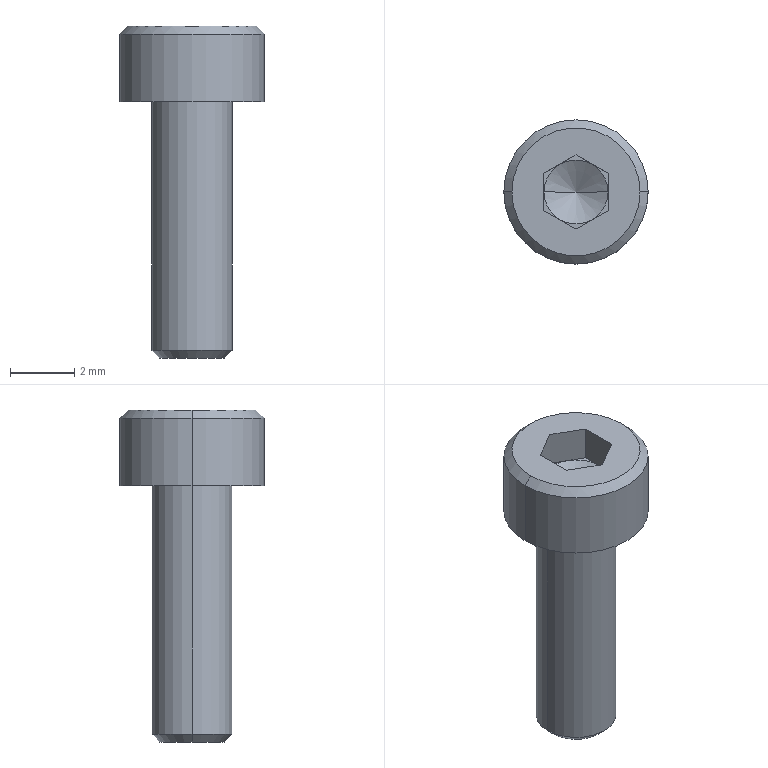Part | SolidWorks | features BaseBody 1 | 1 solid | 25 faces | box 4.5 x 4.5 x 10.36 mm | volume 71.746 mm3 | plane 15 | cone 6 | cylinder 4 | commonest cylinder face diameters 2.5 x2 4.5 x2
STEP:
#1=CARTESIAN_POINT('',(2.15,5.6,3.));
#2=VERTEX_POINT('',#1);
#3=CARTESIAN_POINT('',(4.65,5.6,3.));
#4=VERTEX_POINT('',#3);
#5=CARTESIAN_POINT('',(3.4,5.6,3.));
#6=DIRECTION('',(0.,0.,-1.));
#7=DIRECTION('',(-1.,0.,0.));
#8=AXIS2_PLACEMENT_3D('',#5,#6,#7);
#9=CIRCLE('',#8,1.25);
#10=EDGE_CURVE('',#2,#4,#9,.T.);
#11=ORIENTED_EDGE('',*,*,#10,.T.);
#12=CARTESIAN_POINT('',(4.65,5.6,-4.756));
#13=VERTEX_POINT('',#12);
#14=CARTESIAN_POINT('',(4.65,5.6,-0.8782));
#15=DIRECTION('',(0.,0.,-1.));
#16=VECTOR('',#15,1000.);
#17=LINE('',#14,#16);
#18=EDGE_CURVE('',#4,#13,#17,.T.);
#19=ORIENTED_EDGE('',*,*,#18,.T.);
#20=CARTESIAN_POINT('',(2.15,5.6,-4.756));
#21=VERTEX_POINT('',#20);
#22=CARTESIAN_POINT('',(3.4,5.6,-4.756));
#23=DIRECTION('',(0.,0.,1.));
#24=DIRECTION('',(-1.,0.,0.));
#25=AXIS2_PLACEMENT_3D('',#22,#23,#24);
#26=CIRCLE('',#25,1.25);
#27=EDGE_CURVE('',#13,#21,#26,.T.);
#28=ORIENTED_EDGE('',*,*,#27,.T.);
#29=CARTESIAN_POINT('',(2.15,5.6,-0.8782));
#30=DIRECTION('',(0.,0.,-1.));
#31=VECTOR('',#30,1000.);
#32=LINE('',#29,#31);
#33=EDGE_CURVE('',#2,#21,#32,.T.);
#34=ORIENTED_EDGE('',*,*,#33,.F.);
#35=EDGE_LOOP('',(#11,#19,#28,#34));
#36=FACE_OUTER_BOUND('',#35,.T.);
#37=CARTESIAN_POINT('',(3.4,5.6,-0.8782));
#38=DIRECTION('',(0.,0.,-1.));
#39=DIRECTION('',(-1.,0.,0.));
#40=AXIS2_PLACEMENT_3D('',#37,#38,#39);
#41=CYLINDRICAL_SURFACE('',#40,1.25);
#42=ADVANCED_FACE('',(#36),#41,.T.);
#43=CARTESIAN_POINT('',(4.406,5.6,-5.));
#44=VERTEX_POINT('',#43);
#45=CARTESIAN_POINT('',(2.394,5.6,-5.));
#46=VERTEX_POINT('',#45);
#47=CARTESIAN_POINT('',(3.4,5.6,-5.));
#48=DIRECTION('',(0.,0.,1.));
#49=DIRECTION('',(1.,0.,0.));
#50=AXIS2_PLACEMENT_3D('',#47,#48,#49);
#51=CIRCLE('',#50,1.006);
#52=EDGE_CURVE('',#44,#46,#51,.T.);
#53=ORIENTED_EDGE('',*,*,#52,.T.);
#54=CARTESIAN_POINT('',(2.15,5.6,-4.756));
#55=DIRECTION('',(-0.7071,0.,0.7071));
#56=VECTOR('',#55,1000.);
#57=LINE('',#54,#56);
#58=EDGE_CURVE('',#46,#21,#57,.T.);
#59=ORIENTED_EDGE('',*,*,#58,.T.);
#60=ORIENTED_EDGE('',*,*,#27,.F.);
#61=CARTESIAN_POINT('',(4.65,5.6,-4.756));
#62=DIRECTION('',(0.7071,0.,0.7071));
#63=VECTOR('',#62,1000.);
#64=LINE('',#61,#63);
#65=EDGE_CURVE('',#44,#13,#64,.T.);
#66=ORIENTED_EDGE('',*,*,#65,.F.);
#67=EDGE_LOOP('',(#53,#59,#60,#66));
#68=FACE_OUTER_BOUND('',#67,.T.);
#69=CARTESIAN_POINT('',(3.4,5.6,-4.756));
#70=DIRECTION('',(0.,0.,1.));
#71=DIRECTION('',(1.,0.,0.));
#72=AXIS2_PLACEMENT_3D('',#69,#70,#71);
#73=CONICAL_SURFACE('',#72,1.25,0.7854);
#74=ADVANCED_FACE('',(#68),#73,.T.);
#75=CARTESIAN_POINT('',(1.15,5.6,5.11));
#76=VERTEX_POINT('',#75);
#77=CARTESIAN_POINT('',(5.65,5.6,5.11));
#78=VERTEX_POINT('',#77);
#79=CARTESIAN_POINT('',(3.4,5.6,5.11));
#80=DIRECTION('',(0.,0.,-1.));
#81=DIRECTION('',(-1.,0.,0.));
#82=AXIS2_PLACEMENT_3D('',#79,#80,#81);
#83=CIRCLE('',#82,2.25);
#84=EDGE_CURVE('',#76,#78,#83,.T.);
#85=ORIENTED_EDGE('',*,*,#84,.T.);
#86=CARTESIAN_POINT('',(5.65,5.6,3.));
#87=VERTEX_POINT('',#86);
#88=CARTESIAN_POINT('',(5.65,5.6,4.055));
#89=DIRECTION('',(0.,0.,-1.));
#90=VECTOR('',#89,1000.);
#91=LINE('',#88,#90);
#92=EDGE_CURVE('',#78,#87,#91,.T.);
#93=ORIENTED_EDGE('',*,*,#92,.T.);
#94=CARTESIAN_POINT('',(1.15,5.6,3.));
#95=VERTEX_POINT('',#94);
#96=CARTESIAN_POINT('',(3.4,5.6,3.));
#97=DIRECTION('',(0.,0.,-1.));
#98=DIRECTION('',(-1.,0.,0.));
#99=AXIS2_PLACEMENT_3D('',#96,#97,#98);
#100=CIRCLE('',#99,2.25);
#101=EDGE_CURVE('',#95,#87,#100,.T.);
#102=ORIENTED_EDGE('',*,*,#101,.F.);
#103=CARTESIAN_POINT('',(1.15,5.6,4.055));
#104=DIRECTION('',(0.,0.,-1.));
#105=VECTOR('',#104,1000.);
#106=LINE('',#103,#105);
#107=EDGE_CURVE('',#76,#95,#106,.T.);
#108=ORIENTED_EDGE('',*,*,#107,.F.);
#109=EDGE_LOOP('',(#85,#93,#102,#108));
#110=FACE_OUTER_BOUND('',#109,.T.);
#111=CARTESIAN_POINT('',(3.4,5.6,4.055));
#112=DIRECTION('',(0.,0.,-1.));
#113=DIRECTION('',(-1.,0.,0.));
#114=AXIS2_PLACEMENT_3D('',#111,#112,#113);
#115=CYLINDRICAL_SURFACE('',#114,2.25);
#116=ADVANCED_FACE('',(#110),#115,.T.);
#117=CARTESIAN_POINT('',(1.4,5.6,5.36));
#118=VERTEX_POINT('',#117);
#119=CARTESIAN_POINT('',(5.4,5.6,5.36));
#120=VERTEX_POINT('',#119);
#121=CARTESIAN_POINT('',(3.4,5.6,5.36));
#122=DIRECTION('',(0.,0.,-1.));
#123=DIRECTION('',(-1.,0.,0.));
#124=AXIS2_PLACEMENT_3D('',#121,#122,#123);
#125=CIRCLE('',#124,2.);
#126=EDGE_CURVE('',#118,#120,#125,.T.);
#127=ORIENTED_EDGE('',*,*,#126,.T.);
#128=CARTESIAN_POINT('',(5.65,5.6,5.11));
#129=DIRECTION('',(0.7071,0.,-0.7071));
#130=VECTOR('',#129,1000.);
#131=LINE('',#128,#130);
#132=EDGE_CURVE('',#120,#78,#131,.T.);
#133=ORIENTED_EDGE('',*,*,#132,.T.);
#134=ORIENTED_EDGE('',*,*,#84,.F.);
#135=CARTESIAN_POINT('',(1.15,5.6,5.11));
#136=DIRECTION('',(-0.7071,0.,-0.7071));
#137=VECTOR('',#136,1000.);
#138=LINE('',#135,#137);
#139=EDGE_CURVE('',#118,#76,#138,.T.);
#140=ORIENTED_EDGE('',*,*,#139,.F.);
#141=EDGE_LOOP('',(#127,#133,#134,#140));
#142=FACE_OUTER_BOUND('',#141,.T.);
#143=CARTESIAN_POINT('',(3.4,5.6,5.11));
#144=DIRECTION('',(0.,0.,-1.));
#145=DIRECTION('',(-1.,0.,0.));
#146=AXIS2_PLACEMENT_3D('',#143,#144,#145);
#147=CONICAL_SURFACE('',#146,2.25,0.7854);
#148=ADVANCED_FACE('',(#142),#147,.T.);
#149=CARTESIAN_POINT('',(3.4,5.6,3.683));
#150=VERTEX_POINT('',#149);
#151=CARTESIAN_POINT('',(4.4,5.6,4.26));
#152=VERTEX_POINT('',#151);
#153=CARTESIAN_POINT('',(4.4,5.6,4.26));
#154=DIRECTION('',(0.866,0.,0.5));
#155=VECTOR('',#154,1000.);
#156=LINE('',#153,#155);
#157=EDGE_CURVE('',#150,#152,#156,.T.);
#158=ORIENTED_EDGE('',*,*,#157,.F.);
#159=CARTESIAN_POINT('',(2.4,5.6,4.26));
#160=VERTEX_POINT('',#159);
#161=CARTESIAN_POINT('',(2.4,5.6,4.26));
#162=DIRECTION('',(-0.866,0.,0.5));
#163=VECTOR('',#162,1000.);
#164=LINE('',#161,#163);
#165=EDGE_CURVE('',#150,#160,#164,.T.);
#166=ORIENTED_EDGE('',*,*,#165,.T.);
#167=CARTESIAN_POINT('',(2.9,4.734,4.26));
#168=VERTEX_POINT('',#167);
#169=CARTESIAN_POINT('',(3.4,5.6,4.26));
#170=DIRECTION('',(0.,0.,1.));
#171=DIRECTION('',(1.,0.,0.));
#172=AXIS2_PLACEMENT_3D('',#169,#170,#171);
#173=CIRCLE('',#172,1.);
#174=EDGE_CURVE('',#160,#168,#173,.T.);
#175=ORIENTED_EDGE('',*,*,#174,.T.);
#176=CARTESIAN_POINT('',(3.9,4.734,4.26));
#177=VERTEX_POINT('',#176);
#178=CARTESIAN_POINT('',(3.4,5.6,4.26));
#179=DIRECTION('',(0.,0.,1.));
#180=DIRECTION('',(1.,0.,0.));
#181=AXIS2_PLACEMENT_3D('',#178,#179,#180);
#182=CIRCLE('',#181,1.);
#183=EDGE_CURVE('',#168,#177,#182,.T.);
#184=ORIENTED_EDGE('',*,*,#183,.T.);
#185=CARTESIAN_POINT('',(3.4,5.6,4.26));
#186=DIRECTION('',(0.,0.,1.));
#187=DIRECTION('',(1.,0.,0.));
#188=AXIS2_PLACEMENT_3D('',#185,#186,#187);
#189=CIRCLE('',#188,1.);
#190=EDGE_CURVE('',#177,#152,#189,.T.);
#191=ORIENTED_EDGE('',*,*,#190,.T.);
#192=EDGE_LOOP('',(#158,#166,#175,#184,#191));
#193=FACE_OUTER_BOUND('',#192,.T.);
#194=CARTESIAN_POINT('',(3.4,5.6,4.26));
#195=DIRECTION('',(0.,0.,1.));
#196=DIRECTION('',(1.,0.,0.));
#197=AXIS2_PLACEMENT_3D('',#194,#195,#196);
#198=CONICAL_SURFACE('',#197,1.,1.047);
#199=ADVANCED_FACE('',(#193),#198,.F.);
#200=ORIENTED_EDGE('',*,*,#18,.F.);
#201=CARTESIAN_POINT('',(3.4,5.6,3.));
#202=DIRECTION('',(0.,0.,-1.));
#203=DIRECTION('',(-1.,0.,0.));
#204=AXIS2_PLACEMENT_3D('',#201,#202,#203);
#205=CIRCLE('',#204,1.25);
#206=EDGE_CURVE('',#4,#2,#205,.T.);
#207=ORIENTED_EDGE('',*,*,#206,.T.);
#208=ORIENTED_EDGE('',*,*,#33,.T.);
#209=CARTESIAN_POINT('',(3.4,5.6,-4.756));
#210=DIRECTION('',(0.,0.,1.));
#211=DIRECTION('',(-1.,0.,0.));
#212=AXIS2_PLACEMENT_3D('',#209,#210,#211);
#213=CIRCLE('',#212,1.25);
#214=EDGE_CURVE('',#21,#13,#213,.T.);
#215=ORIENTED_EDGE('',*,*,#214,.T.);
#216=EDGE_LOOP('',(#200,#207,#208,#215));
#217=FACE_OUTER_BOUND('',#216,.T.);
#218=CARTESIAN_POINT('',(3.4,5.6,-0.8782));
#219=DIRECTION('',(0.,0.,-1.));
#220=DIRECTION('',(-1.,0.,0.));
#221=AXIS2_PLACEMENT_3D('',#218,#219,#220);
#222=CYLINDRICAL_SURFACE('',#221,1.25);
#223=ADVANCED_FACE('',(#217),#222,.T.);
#224=ORIENTED_EDGE('',*,*,#10,.F.);
#225=ORIENTED_EDGE('',*,*,#206,.F.);
#226=EDGE_LOOP('',(#224,#225));
#227=FACE_BOUND('',#226,.T.);
#228=ORIENTED_EDGE('',*,*,#101,.T.);
#229=CARTESIAN_POINT('',(3.4,5.6,3.));
#230=DIRECTION('',(0.,0.,-1.));
#231=DIRECTION('',(-1.,0.,0.));
#232=AXIS2_PLACEMENT_3D('',#229,#230,#231);
#233=CIRCLE('',#232,2.25);
#234=EDGE_CURVE('',#87,#95,#233,.T.);
#235=ORIENTED_EDGE('',*,*,#234,.T.);
#236=EDGE_LOOP('',(#228,#235));
#237=FACE_OUTER_BOUND('',#236,.T.);
#238=CARTESIAN_POINT('',(3.4,3.85,3.));
#239=DIRECTION('',(0.,0.,-1.));
#240=DIRECTION('',(-1.,0.,0.));
#241=AXIS2_PLACEMENT_3D('',#238,#239,#240);
#242=PLANE('',#241);
#243=ADVANCED_FACE('',(#227,#237),#242,.T.);
#244=ORIENTED_EDGE('',*,*,#58,.F.);
#245=CARTESIAN_POINT('',(3.4,5.6,-5.));
#246=DIRECTION('',(0.,0.,1.));
#247=DIRECTION('',(1.,0.,0.));
#248=AXIS2_PLACEMENT_3D('',#245,#246,#247);
#249=CIRCLE('',#248,1.006);
#250=EDGE_CURVE('',#46,#44,#249,.T.);
#251=ORIENTED_EDGE('',*,*,#250,.T.);
#252=ORIENTED_EDGE('',*,*,#65,.T.);
#253=ORIENTED_EDGE('',*,*,#214,.F.);
#254=EDGE_LOOP('',(#244,#251,#252,#253));
#255=FACE_OUTER_BOUND('',#254,.T.);
#256=CARTESIAN_POINT('',(3.4,5.6,-4.756));
#257=DIRECTION('',(0.,0.,1.));
#258=DIRECTION('',(1.,0.,0.));
#259=AXIS2_PLACEMENT_3D('',#256,#257,#258);
#260=CONICAL_SURFACE('',#259,1.25,0.7854);
#261=ADVANCED_FACE('',(#255),#260,.T.);
#262=ORIENTED_EDGE('',*,*,#92,.F.);
#263=CARTESIAN_POINT('',(3.4,5.6,5.11));
#264=DIRECTION('',(0.,0.,-1.));
#265=DIRECTION('',(-1.,0.,0.));
#266=AXIS2_PLACEMENT_3D('',#263,#264,#265);
#267=CIRCLE('',#266,2.25);
#268=EDGE_CURVE('',#78,#76,#267,.T.);
#269=ORIENTED_EDGE('',*,*,#268,.T.);
#270=ORIENTED_EDGE('',*,*,#107,.T.);
#271=ORIENTED_EDGE('',*,*,#234,.F.);
#272=EDGE_LOOP('',(#262,#269,#270,#271));
#273=FACE_OUTER_BOUND('',#272,.T.);
#274=CARTESIAN_POINT('',(3.4,5.6,4.055));
#275=DIRECTION('',(0.,0.,-1.));
#276=DIRECTION('',(-1.,0.,0.));
#277=AXIS2_PLACEMENT_3D('',#274,#275,#276);
#278=CYLINDRICAL_SURFACE('',#277,2.25);
#279=ADVANCED_FACE('',(#273),#278,.T.);
#280=ORIENTED_EDGE('',*,*,#52,.F.);
#281=ORIENTED_EDGE('',*,*,#250,.F.);
#282=EDGE_LOOP('',(#280,#281));
#283=FACE_OUTER_BOUND('',#282,.T.);
#284=CARTESIAN_POINT('',(3.4,5.097,-5.));
#285=DIRECTION('',(0.,0.,-1.));
#286=DIRECTION('',(-1.,0.,0.));
#287=AXIS2_PLACEMENT_3D('',#284,#285,#286);
#288=PLANE('',#287);
#289=ADVANCED_FACE('',(#283),#288,.T.);
#290=ORIENTED_EDGE('',*,*,#132,.F.);
#291=CARTESIAN_POINT('',(3.4,5.6,5.36));
#292=DIRECTION('',(0.,0.,-1.));
#293=DIRECTION('',(-1.,0.,0.));
#294=AXIS2_PLACEMENT_3D('',#291,#292,#293);
#295=CIRCLE('',#294,2.);
#296=EDGE_CURVE('',#120,#118,#295,.T.);
#297=ORIENTED_EDGE('',*,*,#296,.T.);
#298=ORIENTED_EDGE('',*,*,#139,.T.);
#299=ORIENTED_EDGE('',*,*,#268,.F.);
#300=EDGE_LOOP('',(#290,#297,#298,#299));
#301=FACE_OUTER_BOUND('',#300,.T.);
#302=CARTESIAN_POINT('',(3.4,5.6,5.11));
#303=DIRECTION('',(0.,0.,-1.));
#304=DIRECTION('',(-1.,0.,0.));
#305=AXIS2_PLACEMENT_3D('',#302,#303,#304);
#306=CONICAL_SURFACE('',#305,2.25,0.7854);
#307=ADVANCED_FACE('',(#301),#306,.T.);
#308=ORIENTED_EDGE('',*,*,#126,.F.);
#309=ORIENTED_EDGE('',*,*,#296,.F.);
#310=EDGE_LOOP('',(#308,#309));
#311=FACE_OUTER_BOUND('',#310,.T.);
#312=CARTESIAN_POINT('',(4.4,6.177,5.36));
#313=VERTEX_POINT('',#312);
#314=CARTESIAN_POINT('',(4.4,5.023,5.36));
#315=VERTEX_POINT('',#314);
#316=CARTESIAN_POINT('',(4.4,4.6,5.36));
#317=DIRECTION('',(0.,-1.,0.));
#318=VECTOR('',#317,1000.);
#319=LINE('',#316,#318);
#320=EDGE_CURVE('',#313,#315,#319,.T.);
#321=ORIENTED_EDGE('',*,*,#320,.T.);
#322=CARTESIAN_POINT('',(3.4,4.445,5.36));
#323=VERTEX_POINT('',#322);
#324=CARTESIAN_POINT('',(4.4,5.023,5.36));
#325=DIRECTION('',(-0.866,-0.5,0.));
#326=VECTOR('',#325,1000.);
#327=LINE('',#324,#326);
#328=EDGE_CURVE('',#315,#323,#327,.T.);
#329=ORIENTED_EDGE('',*,*,#328,.T.);
#330=CARTESIAN_POINT('',(2.4,5.023,5.36));
#331=VERTEX_POINT('',#330);
#332=CARTESIAN_POINT('',(3.4,4.445,5.36));
#333=DIRECTION('',(-0.866,0.5,0.));
#334=VECTOR('',#333,1000.);
#335=LINE('',#332,#334);
#336=EDGE_CURVE('',#323,#331,#335,.T.);
#337=ORIENTED_EDGE('',*,*,#336,.T.);
#338=CARTESIAN_POINT('',(2.4,6.177,5.36));
#339=VERTEX_POINT('',#338);
#340=CARTESIAN_POINT('',(2.4,4.6,5.36));
#341=DIRECTION('',(0.,1.,0.));
#342=VECTOR('',#341,1000.);
#343=LINE('',#340,#342);
#344=EDGE_CURVE('',#331,#339,#343,.T.);
#345=ORIENTED_EDGE('',*,*,#344,.T.);
#346=CARTESIAN_POINT('',(3.4,6.755,5.36));
#347=VERTEX_POINT('',#346);
#348=CARTESIAN_POINT('',(2.4,6.177,5.36));
#349=DIRECTION('',(0.866,0.5,0.));
#350=VECTOR('',#349,1000.);
#351=LINE('',#348,#350);
#352=EDGE_CURVE('',#339,#347,#351,.T.);
#353=ORIENTED_EDGE('',*,*,#352,.T.);
#354=CARTESIAN_POINT('',(3.4,6.755,5.36));
#355=DIRECTION('',(0.866,-0.5,0.));
#356=VECTOR('',#355,1000.);
#357=LINE('',#354,#356);
#358=EDGE_CURVE('',#347,#313,#357,.T.);
#359=ORIENTED_EDGE('',*,*,#358,.T.);
#360=EDGE_LOOP('',(#321,#329,#337,#345,#353,#359));
#361=FACE_BOUND('',#360,.T.);
#362=CARTESIAN_POINT('',(3.4,4.6,5.36));
#363=DIRECTION('',(0.,0.,1.));
#364=DIRECTION('',(1.,0.,0.));
#365=AXIS2_PLACEMENT_3D('',#362,#363,#364);
#366=PLANE('',#365);
#367=ADVANCED_FACE('',(#311,#361),#366,.T.);
#368=CARTESIAN_POINT('',(3.4,4.445,4.26));
#369=VERTEX_POINT('',#368);
#370=CARTESIAN_POINT('',(3.4,4.445,5.36));
#371=DIRECTION('',(0.,0.,-1.));
#372=VECTOR('',#371,1000.);
#373=LINE('',#370,#372);
#374=EDGE_CURVE('',#323,#369,#373,.T.);
#375=ORIENTED_EDGE('',*,*,#374,.F.);
#376=ORIENTED_EDGE('',*,*,#328,.F.);
#377=CARTESIAN_POINT('',(4.4,5.023,4.26));
#378=VERTEX_POINT('',#377);
#379=CARTESIAN_POINT('',(4.4,5.023,5.36));
#380=DIRECTION('',(0.,0.,1.));
#381=VECTOR('',#380,1000.);
#382=LINE('',#379,#381);
#383=EDGE_CURVE('',#378,#315,#382,.T.);
#384=ORIENTED_EDGE('',*,*,#383,.F.);
#385=CARTESIAN_POINT('',(3.4,4.445,4.26));
#386=DIRECTION('',(0.866,0.5,0.));
#387=VECTOR('',#386,1000.);
#388=LINE('',#385,#387);
#389=EDGE_CURVE('',#177,#378,#388,.T.);
#390=ORIENTED_EDGE('',*,*,#389,.F.);
#391=CARTESIAN_POINT('',(3.4,4.445,4.26));
#392=DIRECTION('',(0.866,0.5,0.));
#393=VECTOR('',#392,1000.);
#394=LINE('',#391,#393);
#395=EDGE_CURVE('',#369,#177,#394,.T.);
#396=ORIENTED_EDGE('',*,*,#395,.F.);
#397=EDGE_LOOP('',(#375,#376,#384,#390,#396));
#398=FACE_OUTER_BOUND('',#397,.T.);
#399=CARTESIAN_POINT('',(3.4,4.445,5.36));
#400=DIRECTION('',(0.5,-0.866,0.));
#401=DIRECTION('',(0.866,0.5,0.));
#402=AXIS2_PLACEMENT_3D('',#399,#400,#401);
#403=PLANE('',#402);
#404=ADVANCED_FACE('',(#398),#403,.F.);
#405=ORIENTED_EDGE('',*,*,#383,.T.);
#406=ORIENTED_EDGE('',*,*,#320,.F.);
#407=CARTESIAN_POINT('',(4.4,6.177,4.26));
#408=VERTEX_POINT('',#407);
#409=CARTESIAN_POINT('',(4.4,6.177,5.36));
#410=DIRECTION('',(0.,0.,1.));
#411=VECTOR('',#410,1000.);
#412=LINE('',#409,#411);
#413=EDGE_CURVE('',#408,#313,#412,.T.);
#414=ORIENTED_EDGE('',*,*,#413,.F.);
#415=CARTESIAN_POINT('',(4.4,5.023,4.26));
#416=DIRECTION('',(0.,1.,0.));
#417=VECTOR('',#416,1000.);
#418=LINE('',#415,#417);
#419=EDGE_CURVE('',#152,#408,#418,.T.);
#420=ORIENTED_EDGE('',*,*,#419,.F.);
#421=CARTESIAN_POINT('',(4.4,5.023,4.26));
#422=DIRECTION('',(0.,1.,0.));
#423=VECTOR('',#422,1000.);
#424=LINE('',#421,#423);
#425=EDGE_CURVE('',#378,#152,#424,.T.);
#426=ORIENTED_EDGE('',*,*,#425,.F.);
#427=EDGE_LOOP('',(#405,#406,#414,#420,#426));
#428=FACE_OUTER_BOUND('',#427,.T.);
#429=CARTESIAN_POINT('',(4.4,5.023,5.36));
#430=DIRECTION('',(1.,0.,0.));
#431=DIRECTION('',(0.,0.,-1.));
#432=AXIS2_PLACEMENT_3D('',#429,#430,#431);
#433=PLANE('',#432);
#434=ADVANCED_FACE('',(#428),#433,.F.);
#435=ORIENTED_EDGE('',*,*,#413,.T.);
#436=ORIENTED_EDGE('',*,*,#358,.F.);
#437=CARTESIAN_POINT('',(3.4,6.755,4.26));
#438=VERTEX_POINT('',#437);
#439=CARTESIAN_POINT('',(3.4,6.755,5.36));
#440=DIRECTION('',(0.,0.,1.));
#441=VECTOR('',#440,1000.);
#442=LINE('',#439,#441);
#443=EDGE_CURVE('',#438,#347,#442,.T.);
#444=ORIENTED_EDGE('',*,*,#443,.F.);
#445=CARTESIAN_POINT('',(3.9,6.466,4.26));
#446=VERTEX_POINT('',#445);
#447=CARTESIAN_POINT('',(4.4,6.177,4.26));
#448=DIRECTION('',(-0.866,0.5,0.));
#449=VECTOR('',#448,1000.);
#450=LINE('',#447,#449);
#451=EDGE_CURVE('',#446,#438,#450,.T.);
#452=ORIENTED_EDGE('',*,*,#451,.F.);
#453=CARTESIAN_POINT('',(4.4,6.177,4.26));
#454=DIRECTION('',(-0.866,0.5,0.));
#455=VECTOR('',#454,1000.);
#456=LINE('',#453,#455);
#457=EDGE_CURVE('',#408,#446,#456,.T.);
#458=ORIENTED_EDGE('',*,*,#457,.F.);
#459=EDGE_LOOP('',(#435,#436,#444,#452,#458));
#460=FACE_OUTER_BOUND('',#459,.T.);
#461=CARTESIAN_POINT('',(4.4,6.177,5.36));
#462=DIRECTION('',(0.5,0.866,0.));
#463=DIRECTION('',(-0.866,0.5,0.));
#464=AXIS2_PLACEMENT_3D('',#461,#462,#463);
#465=PLANE('',#464);
#466=ADVANCED_FACE('',(#460),#465,.F.);
#467=ORIENTED_EDGE('',*,*,#443,.T.);
#468=ORIENTED_EDGE('',*,*,#352,.F.);
#469=CARTESIAN_POINT('',(2.4,6.177,4.26));
#470=VERTEX_POINT('',#469);
#471=CARTESIAN_POINT('',(2.4,6.177,5.36));
#472=DIRECTION('',(0.,0.,1.));
#473=VECTOR('',#472,1000.);
#474=LINE('',#471,#473);
#475=EDGE_CURVE('',#470,#339,#474,.T.);
#476=ORIENTED_EDGE('',*,*,#475,.F.);
#477=CARTESIAN_POINT('',(2.9,6.466,4.26));
#478=VERTEX_POINT('',#477);
#479=CARTESIAN_POINT('',(3.4,6.755,4.26));
#480=DIRECTION('',(-0.866,-0.5,0.));
#481=VECTOR('',#480,1000.);
#482=LINE('',#479,#481);
#483=EDGE_CURVE('',#478,#470,#482,.T.);
#484=ORIENTED_EDGE('',*,*,#483,.F.);
#485=CARTESIAN_POINT('',(3.4,6.755,4.26));
#486=DIRECTION('',(-0.866,-0.5,0.));
#487=VECTOR('',#486,1000.);
#488=LINE('',#485,#487);
#489=EDGE_CURVE('',#438,#478,#488,.T.);
#490=ORIENTED_EDGE('',*,*,#489,.F.);
#491=EDGE_LOOP('',(#467,#468,#476,#484,#490));
#492=FACE_OUTER_BOUND('',#491,.T.);
#493=CARTESIAN_POINT('',(3.4,6.755,5.36));
#494=DIRECTION('',(-0.5,0.866,0.));
#495=DIRECTION('',(-0.866,-0.5,0.));
#496=AXIS2_PLACEMENT_3D('',#493,#494,#495);
#497=PLANE('',#496);
#498=ADVANCED_FACE('',(#492),#497,.F.);
#499=ORIENTED_EDGE('',*,*,#475,.T.);
#500=ORIENTED_EDGE('',*,*,#344,.F.);
#501=CARTESIAN_POINT('',(2.4,5.023,4.26));
#502=VERTEX_POINT('',#501);
#503=CARTESIAN_POINT('',(2.4,5.023,5.36));
#504=DIRECTION('',(0.,0.,1.));
#505=VECTOR('',#504,1000.);
#506=LINE('',#503,#505);
#507=EDGE_CURVE('',#502,#331,#506,.T.);
#508=ORIENTED_EDGE('',*,*,#507,.F.);
#509=CARTESIAN_POINT('',(2.4,6.177,4.26));
#510=DIRECTION('',(0.,-1.,0.));
#511=VECTOR('',#510,1000.);
#512=LINE('',#509,#511);
#513=EDGE_CURVE('',#160,#502,#512,.T.);
#514=ORIENTED_EDGE('',*,*,#513,.F.);
#515=CARTESIAN_POINT('',(2.4,6.177,4.26));
#516=DIRECTION('',(0.,-1.,0.));
#517=VECTOR('',#516,1000.);
#518=LINE('',#515,#517);
#519=EDGE_CURVE('',#470,#160,#518,.T.);
#520=ORIENTED_EDGE('',*,*,#519,.F.);
#521=EDGE_LOOP('',(#499,#500,#508,#514,#520));
#522=FACE_OUTER_BOUND('',#521,.T.);
#523=CARTESIAN_POINT('',(2.4,6.177,5.36));
#524=DIRECTION('',(-1.,0.,0.));
#525=DIRECTION('',(0.,0.,1.));
#526=AXIS2_PLACEMENT_3D('',#523,#524,#525);
#527=PLANE('',#526);
#528=ADVANCED_FACE('',(#522),#527,.F.);
#529=ORIENTED_EDGE('',*,*,#507,.T.);
#530=ORIENTED_EDGE('',*,*,#336,.F.);
#531=ORIENTED_EDGE('',*,*,#374,.T.);
#532=CARTESIAN_POINT('',(2.4,5.023,4.26));
#533=DIRECTION('',(0.866,-0.5,0.));
#534=VECTOR('',#533,1000.);
#535=LINE('',#532,#534);
#536=EDGE_CURVE('',#168,#369,#535,.T.);
#537=ORIENTED_EDGE('',*,*,#536,.F.);
#538=CARTESIAN_POINT('',(2.4,5.023,4.26));
#539=DIRECTION('',(0.866,-0.5,0.));
#540=VECTOR('',#539,1000.);
#541=LINE('',#538,#540);
#542=EDGE_CURVE('',#502,#168,#541,.T.);
#543=ORIENTED_EDGE('',*,*,#542,.F.);
#544=EDGE_LOOP('',(#529,#530,#531,#537,#543));
#545=FACE_OUTER_BOUND('',#544,.T.);
#546=CARTESIAN_POINT('',(2.4,5.023,5.36));
#547=DIRECTION('',(-0.5,-0.866,0.));
#548=DIRECTION('',(0.866,-0.5,0.));
#549=AXIS2_PLACEMENT_3D('',#546,#547,#548);
#550=PLANE('',#549);
#551=ADVANCED_FACE('',(#545),#550,.F.);
#552=ORIENTED_EDGE('',*,*,#183,.F.);
#553=ORIENTED_EDGE('',*,*,#536,.T.);
#554=ORIENTED_EDGE('',*,*,#395,.T.);
#555=EDGE_LOOP('',(#552,#553,#554));
#556=FACE_OUTER_BOUND('',#555,.T.);
#557=CARTESIAN_POINT('',(3.4,5.6,4.26));
#558=DIRECTION('',(0.,0.,-1.));
#559=DIRECTION('',(-1.,0.,0.));
#560=AXIS2_PLACEMENT_3D('',#557,#558,#559);
#561=PLANE('',#560);
#562=ADVANCED_FACE('',(#556),#561,.F.);
#563=ORIENTED_EDGE('',*,*,#389,.T.);
#564=ORIENTED_EDGE('',*,*,#425,.T.);
#565=ORIENTED_EDGE('',*,*,#190,.F.);
#566=EDGE_LOOP('',(#563,#564,#565));
#567=FACE_OUTER_BOUND('',#566,.T.);
#568=CARTESIAN_POINT('',(3.4,5.6,4.26));
#569=DIRECTION('',(0.,0.,-1.));
#570=DIRECTION('',(-1.,0.,0.));
#571=AXIS2_PLACEMENT_3D('',#568,#569,#570);
#572=PLANE('',#571);
#573=ADVANCED_FACE('',(#567),#572,.F.);
#574=ORIENTED_EDGE('',*,*,#419,.T.);
#575=ORIENTED_EDGE('',*,*,#457,.T.);
#576=CARTESIAN_POINT('',(3.4,5.6,4.26));
#577=DIRECTION('',(0.,0.,1.));
#578=DIRECTION('',(1.,0.,0.));
#579=AXIS2_PLACEMENT_3D('',#576,#577,#578);
#580=CIRCLE('',#579,1.);
#581=EDGE_CURVE('',#152,#446,#580,.T.);
#582=ORIENTED_EDGE('',*,*,#581,.F.);
#583=EDGE_LOOP('',(#574,#575,#582));
#584=FACE_OUTER_BOUND('',#583,.T.);
#585=CARTESIAN_POINT('',(3.4,5.6,4.26));
#586=DIRECTION('',(0.,0.,-1.));
#587=DIRECTION('',(-1.,0.,0.));
#588=AXIS2_PLACEMENT_3D('',#585,#586,#587);
#589=PLANE('',#588);
#590=ADVANCED_FACE('',(#584),#589,.F.);
#591=CARTESIAN_POINT('',(3.4,5.6,4.26));
#592=DIRECTION('',(0.,0.,1.));
#593=DIRECTION('',(1.,0.,0.));
#594=AXIS2_PLACEMENT_3D('',#591,#592,#593);
#595=CIRCLE('',#594,1.);
#596=EDGE_CURVE('',#446,#478,#595,.T.);
#597=ORIENTED_EDGE('',*,*,#596,.F.);
#598=ORIENTED_EDGE('',*,*,#451,.T.);
#599=ORIENTED_EDGE('',*,*,#489,.T.);
#600=EDGE_LOOP('',(#597,#598,#599));
#601=FACE_OUTER_BOUND('',#600,.T.);
#602=CARTESIAN_POINT('',(3.4,5.6,4.26));
#603=DIRECTION('',(0.,0.,-1.));
#604=DIRECTION('',(-1.,0.,0.));
#605=AXIS2_PLACEMENT_3D('',#602,#603,#604);
#606=PLANE('',#605);
#607=ADVANCED_FACE('',(#601),#606,.F.);
#608=ORIENTED_EDGE('',*,*,#483,.T.);
#609=ORIENTED_EDGE('',*,*,#519,.T.);
#610=CARTESIAN_POINT('',(3.4,5.6,4.26));
#611=DIRECTION('',(0.,0.,1.));
#612=DIRECTION('',(1.,0.,0.));
#613=AXIS2_PLACEMENT_3D('',#610,#611,#612);
#614=CIRCLE('',#613,1.);
#615=EDGE_CURVE('',#478,#160,#614,.T.);
#616=ORIENTED_EDGE('',*,*,#615,.F.);
#617=EDGE_LOOP('',(#608,#609,#616));
#618=FACE_OUTER_BOUND('',#617,.T.);
#619=CARTESIAN_POINT('',(3.4,5.6,4.26));
#620=DIRECTION('',(0.,0.,-1.));
#621=DIRECTION('',(-1.,0.,0.));
#622=AXIS2_PLACEMENT_3D('',#619,#620,#621);
#623=PLANE('',#622);
#624=ADVANCED_FACE('',(#618),#623,.F.);
#625=ORIENTED_EDGE('',*,*,#513,.T.);
#626=ORIENTED_EDGE('',*,*,#542,.T.);
#627=ORIENTED_EDGE('',*,*,#174,.F.);
#628=EDGE_LOOP('',(#625,#626,#627));
#629=FACE_OUTER_BOUND('',#628,.T.);
#630=CARTESIAN_POINT('',(3.4,5.6,4.26));
#631=DIRECTION('',(0.,0.,-1.));
#632=DIRECTION('',(-1.,0.,0.));
#633=AXIS2_PLACEMENT_3D('',#630,#631,#632);
#634=PLANE('',#633);
#635=ADVANCED_FACE('',(#629),#634,.F.);
#636=ORIENTED_EDGE('',*,*,#165,.F.);
#637=ORIENTED_EDGE('',*,*,#157,.T.);
#638=ORIENTED_EDGE('',*,*,#581,.T.);
#639=ORIENTED_EDGE('',*,*,#596,.T.);
#640=ORIENTED_EDGE('',*,*,#615,.T.);
#641=EDGE_LOOP('',(#636,#637,#638,#639,#640));
#642=FACE_OUTER_BOUND('',#641,.T.);
#643=CARTESIAN_POINT('',(3.4,5.6,4.26));
#644=DIRECTION('',(0.,0.,1.));
#645=DIRECTION('',(1.,0.,0.));
#646=AXIS2_PLACEMENT_3D('',#643,#644,#645);
#647=CONICAL_SURFACE('',#646,1.,1.047);
#648=ADVANCED_FACE('',(#642),#647,.F.);
#649=CLOSED_SHELL('',(#42,#74,#116,#148,#199,#223,#243,#261,#279,#289,#307,#367,#404,#434,#466,#498,#528,#551,#562,#573,#590,#607,#624,#635,#648));
#650=MANIFOLD_SOLID_BREP('',#649);
#651=CARTESIAN_POINT('',(0.,0.,0.));
#652=DIRECTION('',(0.,0.,1.));
#653=DIRECTION('',(1.,0.,0.));
#654=AXIS2_PLACEMENT_3D('',#651,#652,#653);
#655=(LENGTH_UNIT()NAMED_UNIT(*)SI_UNIT(.MILLI.,.METRE.));
#656=UNCERTAINTY_MEASURE_WITH_UNIT(LENGTH_MEASURE(0.00001),#655,'','');
#657=(NAMED_UNIT(*)PLANE_ANGLE_UNIT()SI_UNIT($,.RADIAN.));
#658=(NAMED_UNIT(*)SI_UNIT($,.STERADIAN.)SOLID_ANGLE_UNIT());
#659=(GEOMETRIC_REPRESENTATION_CONTEXT(3)GLOBAL_UNCERTAINTY_ASSIGNED_CONTEXT((#656))GLOBAL_UNIT_ASSIGNED_CONTEXT((#655,#657,#658))REPRESENTATION_CONTEXT('',''));
#660=ADVANCED_BREP_SHAPE_REPRESENTATION('',(#650,#654),#659);